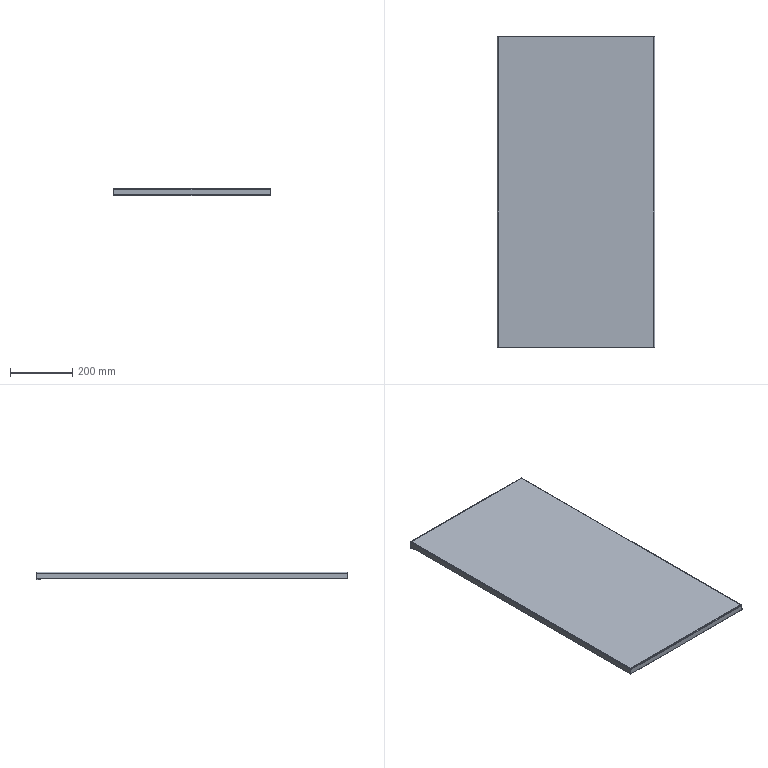Part | SolidWorks | features EdgeFlange 2, CornerFeat 1, FlatPattern 1, ICE 1, SMBaseFlange 1, SheetMetal 1 | 1 solid | 48 faces | box 505 x 1000 x 25 mm | volume 849677 mm3 | plane 30 | cylinder 10 | spline 8 | commonest cylinder face diameters 3 x5 6 x5